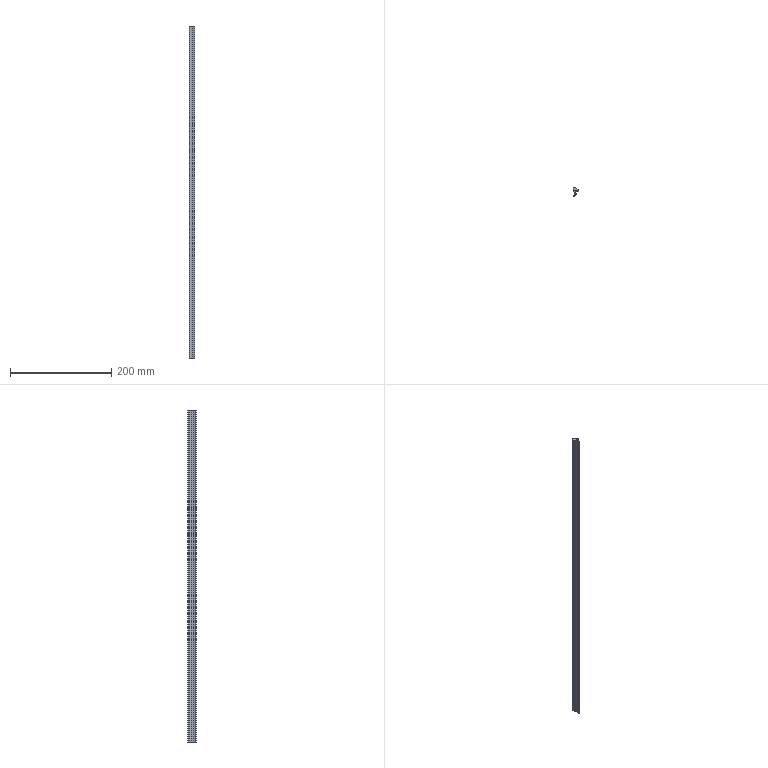Part | SolidWorks | features BaseBody 1, MoveFace 1 | 1 solid | 20 faces | box 10.8 x 17.5 x 657 mm | volume 51772 mm3 | cylinder 11 | plane 9 | commonest cylinder face diameters 1.6 x2 14 x2 0.4 x1 0.6 x1 0.8 x1 2.6 x1
STEP:
#1=CARTESIAN_POINT('',(-3.236,-11.055,557.));
#2=VERTEX_POINT('',#1);
#3=CARTESIAN_POINT('',(-4.3,-10.3,557.));
#4=VERTEX_POINT('',#3);
#5=CARTESIAN_POINT('',(-3.5,-10.3,557.));
#6=DIRECTION('',(0.,0.,-1.));
#7=DIRECTION('',(1.,0.,0.));
#8=AXIS2_PLACEMENT_3D('',#5,#6,#7);
#9=CIRCLE('',#8,0.8);
#10=EDGE_CURVE('',#2,#4,#9,.T.);
#11=ORIENTED_EDGE('',*,*,#10,.T.);
#12=CARTESIAN_POINT('',(-4.3,-10.3,-100.));
#13=VERTEX_POINT('',#12);
#14=CARTESIAN_POINT('',(-4.3,-10.3,-100.));
#15=DIRECTION('',(0.,0.,-1.));
#16=VECTOR('',#15,1000.);
#17=LINE('',#14,#16);
#18=EDGE_CURVE('',#4,#13,#17,.T.);
#19=ORIENTED_EDGE('',*,*,#18,.T.);
#20=CARTESIAN_POINT('',(-3.236,-11.055,-100.));
#21=VERTEX_POINT('',#20);
#22=CARTESIAN_POINT('',(-3.5,-10.3,-100.));
#23=DIRECTION('',(0.,0.,1.));
#24=DIRECTION('',(-1.,0.,0.));
#25=AXIS2_PLACEMENT_3D('',#22,#23,#24);
#26=CIRCLE('',#25,0.8);
#27=EDGE_CURVE('',#13,#21,#26,.T.);
#28=ORIENTED_EDGE('',*,*,#27,.T.);
#29=CARTESIAN_POINT('',(-3.236,-11.055,-100.));
#30=DIRECTION('',(0.,0.,-1.));
#31=VECTOR('',#30,1000.);
#32=LINE('',#29,#31);
#33=EDGE_CURVE('',#2,#21,#32,.T.);
#34=ORIENTED_EDGE('',*,*,#33,.F.);
#35=EDGE_LOOP('',(#11,#19,#28,#34));
#36=FACE_OUTER_BOUND('',#35,.T.);
#37=CARTESIAN_POINT('',(-3.5,-10.3,-100.));
#38=DIRECTION('',(0.,0.,-1.));
#39=DIRECTION('',(-1.,0.,0.));
#40=AXIS2_PLACEMENT_3D('',#37,#38,#39);
#41=CYLINDRICAL_SURFACE('',#40,0.8);
#42=ADVANCED_FACE('',(#36),#41,.T.);
#43=CARTESIAN_POINT('',(1.184,-6.397,-100.));
#44=VERTEX_POINT('',#43);
#45=CARTESIAN_POINT('',(-5.702,-4.29,-100.));
#46=DIRECTION('',(0.,0.,1.));
#47=DIRECTION('',(-1.,0.,0.));
#48=AXIS2_PLACEMENT_3D('',#45,#46,#47);
#49=CIRCLE('',#48,7.201);
#50=EDGE_CURVE('',#21,#44,#49,.T.);
#51=ORIENTED_EDGE('',*,*,#50,.T.);
#52=CARTESIAN_POINT('',(1.184,-6.397,557.));
#53=VERTEX_POINT('',#52);
#54=CARTESIAN_POINT('',(1.184,-6.397,-100.));
#55=DIRECTION('',(0.,0.,1.));
#56=VECTOR('',#55,1000.);
#57=LINE('',#54,#56);
#58=EDGE_CURVE('',#44,#53,#57,.T.);
#59=ORIENTED_EDGE('',*,*,#58,.T.);
#60=CARTESIAN_POINT('',(-5.702,-4.29,557.));
#61=DIRECTION('',(0.,0.,-1.));
#62=DIRECTION('',(1.,0.,0.));
#63=AXIS2_PLACEMENT_3D('',#60,#61,#62);
#64=CIRCLE('',#63,7.201);
#65=EDGE_CURVE('',#53,#2,#64,.T.);
#66=ORIENTED_EDGE('',*,*,#65,.T.);
#67=ORIENTED_EDGE('',*,*,#33,.T.);
#68=EDGE_LOOP('',(#51,#59,#66,#67));
#69=FACE_OUTER_BOUND('',#68,.T.);
#70=CARTESIAN_POINT('',(-5.702,-4.29,-100.));
#71=DIRECTION('',(0.,0.,-1.));
#72=DIRECTION('',(-1.,0.,0.));
#73=AXIS2_PLACEMENT_3D('',#70,#71,#72);
#74=CYLINDRICAL_SURFACE('',#73,7.201);
#75=ADVANCED_FACE('',(#69),#74,.T.);
#76=CARTESIAN_POINT('',(0.9,-6.,-100.));
#77=VERTEX_POINT('',#76);
#78=CARTESIAN_POINT('',(0.9,-6.3,-100.));
#79=DIRECTION('',(0.,0.,1.));
#80=DIRECTION('',(-1.,0.,0.));
#81=AXIS2_PLACEMENT_3D('',#78,#79,#80);
#82=CIRCLE('',#81,0.3);
#83=EDGE_CURVE('',#44,#77,#82,.T.);
#84=ORIENTED_EDGE('',*,*,#83,.T.);
#85=CARTESIAN_POINT('',(0.9,-6.,557.));
#86=VERTEX_POINT('',#85);
#87=CARTESIAN_POINT('',(0.9,-6.,-100.));
#88=DIRECTION('',(0.,0.,1.));
#89=VECTOR('',#88,1000.);
#90=LINE('',#87,#89);
#91=EDGE_CURVE('',#77,#86,#90,.T.);
#92=ORIENTED_EDGE('',*,*,#91,.T.);
#93=CARTESIAN_POINT('',(0.9,-6.3,557.));
#94=DIRECTION('',(0.,0.,-1.));
#95=DIRECTION('',(1.,0.,0.));
#96=AXIS2_PLACEMENT_3D('',#93,#94,#95);
#97=CIRCLE('',#96,0.3);
#98=EDGE_CURVE('',#86,#53,#97,.T.);
#99=ORIENTED_EDGE('',*,*,#98,.T.);
#100=ORIENTED_EDGE('',*,*,#58,.F.);
#101=EDGE_LOOP('',(#84,#92,#99,#100));
#102=FACE_OUTER_BOUND('',#101,.T.);
#103=CARTESIAN_POINT('',(0.9,-6.3,-100.));
#104=DIRECTION('',(0.,0.,-1.));
#105=DIRECTION('',(-1.,0.,0.));
#106=AXIS2_PLACEMENT_3D('',#103,#104,#105);
#107=CYLINDRICAL_SURFACE('',#106,0.3);
#108=ADVANCED_FACE('',(#102),#107,.T.);
#109=CARTESIAN_POINT('',(-2.5,-0.5,-100.));
#110=VERTEX_POINT('',#109);
#111=CARTESIAN_POINT('',(-2.5,-6.153,-100.));
#112=VERTEX_POINT('',#111);
#113=CARTESIAN_POINT('',(-2.5,-6.397,-100.));
#114=DIRECTION('',(0.,-1.,0.));
#115=VECTOR('',#114,1000.);
#116=LINE('',#113,#115);
#117=EDGE_CURVE('',#110,#112,#116,.T.);
#118=ORIENTED_EDGE('',*,*,#117,.F.);
#119=CARTESIAN_POINT('',(-4.2,1.695,-100.));
#120=VERTEX_POINT('',#119);
#121=CARTESIAN_POINT('',(-1.701,1.875,-100.));
#122=DIRECTION('',(0.,0.,1.));
#123=DIRECTION('',(-1.,0.,0.));
#124=AXIS2_PLACEMENT_3D('',#121,#122,#123);
#125=CIRCLE('',#124,2.506);
#126=EDGE_CURVE('',#120,#110,#125,.T.);
#127=ORIENTED_EDGE('',*,*,#126,.F.);
#128=CARTESIAN_POINT('',(-4.2,5.1,-100.));
#129=VERTEX_POINT('',#128);
#130=CARTESIAN_POINT('',(-4.2,-6.397,-100.));
#131=DIRECTION('',(0.,-1.,0.));
#132=VECTOR('',#131,1000.);
#133=LINE('',#130,#132);
#134=EDGE_CURVE('',#129,#120,#133,.T.);
#135=ORIENTED_EDGE('',*,*,#134,.F.);
#136=CARTESIAN_POINT('',(-2.892,6.4,-100.));
#137=VERTEX_POINT('',#136);
#138=CARTESIAN_POINT('',(-2.9,5.1,-100.));
#139=DIRECTION('',(0.,0.,1.));
#140=DIRECTION('',(-1.,0.,0.));
#141=AXIS2_PLACEMENT_3D('',#138,#139,#140);
#142=CIRCLE('',#141,1.3);
#143=EDGE_CURVE('',#137,#129,#142,.T.);
#144=ORIENTED_EDGE('',*,*,#143,.F.);
#145=CARTESIAN_POINT('',(0.5,5.5,-100.));
#146=VERTEX_POINT('',#145);
#147=CARTESIAN_POINT('',(-2.934,-0.5999,-100.));
#148=DIRECTION('',(0.,0.,1.));
#149=DIRECTION('',(-1.,0.,0.));
#150=AXIS2_PLACEMENT_3D('',#147,#148,#149);
#151=CIRCLE('',#150,7.);
#152=EDGE_CURVE('',#146,#137,#151,.T.);
#153=ORIENTED_EDGE('',*,*,#152,.F.);
#154=CARTESIAN_POINT('',(5.5,1.7,-100.));
#155=VERTEX_POINT('',#154);
#156=CARTESIAN_POINT('',(5.5,1.7,-100.));
#157=DIRECTION('',(-0.7962,0.6051,0.));
#158=VECTOR('',#157,1000.);
#159=LINE('',#156,#158);
#160=EDGE_CURVE('',#155,#146,#159,.T.);
#161=ORIENTED_EDGE('',*,*,#160,.F.);
#162=CARTESIAN_POINT('',(6.458,-0.2215,-100.));
#163=VERTEX_POINT('',#162);
#164=CARTESIAN_POINT('',(6.458,-0.2215,-100.));
#165=DIRECTION('',(-0.4462,0.8949,0.));
#166=VECTOR('',#165,1000.);
#167=LINE('',#164,#166);
#168=EDGE_CURVE('',#163,#155,#167,.T.);
#169=ORIENTED_EDGE('',*,*,#168,.F.);
#170=CARTESIAN_POINT('',(5.895,-0.7433,-100.));
#171=VERTEX_POINT('',#170);
#172=CARTESIAN_POINT('',(6.1,-0.4,-100.));
#173=DIRECTION('',(0.,0.,1.));
#174=DIRECTION('',(-1.,0.,0.));
#175=AXIS2_PLACEMENT_3D('',#172,#173,#174);
#176=CIRCLE('',#175,0.4);
#177=EDGE_CURVE('',#171,#163,#176,.T.);
#178=ORIENTED_EDGE('',*,*,#177,.F.);
#179=CARTESIAN_POINT('',(3.,0.,-100.));
#180=VERTEX_POINT('',#179);
#181=CARTESIAN_POINT('',(2.746,-6.995,-100.));
#182=DIRECTION('',(0.,0.,-1.));
#183=DIRECTION('',(-1.,0.,0.));
#184=AXIS2_PLACEMENT_3D('',#181,#182,#183);
#185=CIRCLE('',#184,7.);
#186=EDGE_CURVE('',#180,#171,#185,.T.);
#187=ORIENTED_EDGE('',*,*,#186,.F.);
#188=CARTESIAN_POINT('',(0.,0.,-100.));
#189=VERTEX_POINT('',#188);
#190=CARTESIAN_POINT('',(-6.814,0.,-100.));
#191=DIRECTION('',(1.,0.,0.));
#192=VECTOR('',#191,1000.);
#193=LINE('',#190,#192);
#194=EDGE_CURVE('',#189,#180,#193,.T.);
#195=ORIENTED_EDGE('',*,*,#194,.F.);
#196=CARTESIAN_POINT('',(0.,-5.8,-100.));
#197=VERTEX_POINT('',#196);
#198=CARTESIAN_POINT('',(0.,-6.397,-100.));
#199=DIRECTION('',(0.,1.,0.));
#200=VECTOR('',#199,1000.);
#201=LINE('',#198,#200);
#202=EDGE_CURVE('',#197,#189,#201,.T.);
#203=ORIENTED_EDGE('',*,*,#202,.F.);
#204=CARTESIAN_POINT('',(0.2,-6.,-100.));
#205=VERTEX_POINT('',#204);
#206=CARTESIAN_POINT('',(0.2,-5.8,-100.));
#207=DIRECTION('',(0.,0.,1.));
#208=DIRECTION('',(-1.,0.,0.));
#209=AXIS2_PLACEMENT_3D('',#206,#207,#208);
#210=CIRCLE('',#209,0.2);
#211=EDGE_CURVE('',#197,#205,#210,.T.);
#212=ORIENTED_EDGE('',*,*,#211,.T.);
#213=CARTESIAN_POINT('',(-6.814,-6.,-100.));
#214=DIRECTION('',(-1.,0.,0.));
#215=VECTOR('',#214,1000.);
#216=LINE('',#213,#215);
#217=EDGE_CURVE('',#77,#205,#216,.T.);
#218=ORIENTED_EDGE('',*,*,#217,.F.);
#219=ORIENTED_EDGE('',*,*,#83,.F.);
#220=ORIENTED_EDGE('',*,*,#50,.F.);
#221=ORIENTED_EDGE('',*,*,#27,.F.);
#222=CARTESIAN_POINT('',(-3.998,-9.674,-100.));
#223=VERTEX_POINT('',#222);
#224=CARTESIAN_POINT('',(-3.5,-10.3,-100.));
#225=DIRECTION('',(0.,0.,1.));
#226=DIRECTION('',(-1.,0.,0.));
#227=AXIS2_PLACEMENT_3D('',#224,#225,#226);
#228=CIRCLE('',#227,0.8);
#229=EDGE_CURVE('',#223,#13,#228,.T.);
#230=ORIENTED_EDGE('',*,*,#229,.F.);
#231=CARTESIAN_POINT('',(-6.814,-6.397,-100.));
#232=DIRECTION('',(0.,0.,-1.));
#233=DIRECTION('',(-1.,0.,0.));
#234=AXIS2_PLACEMENT_3D('',#231,#232,#233);
#235=CIRCLE('',#234,4.321);
#236=EDGE_CURVE('',#112,#223,#235,.T.);
#237=ORIENTED_EDGE('',*,*,#236,.F.);
#238=EDGE_LOOP('',(#118,#127,#135,#144,#153,#161,#169,#178,#187,#195,#203,#212,#218,#219,#220,#221,#230,#237));
#239=FACE_OUTER_BOUND('',#238,.T.);
#240=CARTESIAN_POINT('',(-6.814,-6.397,-100.));
#241=DIRECTION('',(0.,0.,1.));
#242=DIRECTION('',(1.,0.,0.));
#243=AXIS2_PLACEMENT_3D('',#240,#241,#242);
#244=PLANE('',#243);
#245=ADVANCED_FACE('',(#239),#244,.F.);
#246=ORIENTED_EDGE('',*,*,#18,.F.);
#247=CARTESIAN_POINT('',(-3.998,-9.674,557.));
#248=VERTEX_POINT('',#247);
#249=CARTESIAN_POINT('',(-3.5,-10.3,557.));
#250=DIRECTION('',(0.,0.,-1.));
#251=DIRECTION('',(1.,0.,0.));
#252=AXIS2_PLACEMENT_3D('',#249,#250,#251);
#253=CIRCLE('',#252,0.8);
#254=EDGE_CURVE('',#4,#248,#253,.T.);
#255=ORIENTED_EDGE('',*,*,#254,.T.);
#256=CARTESIAN_POINT('',(-3.998,-9.674,-100.));
#257=DIRECTION('',(0.,0.,-1.));
#258=VECTOR('',#257,1000.);
#259=LINE('',#256,#258);
#260=EDGE_CURVE('',#248,#223,#259,.T.);
#261=ORIENTED_EDGE('',*,*,#260,.T.);
#262=ORIENTED_EDGE('',*,*,#229,.T.);
#263=EDGE_LOOP('',(#246,#255,#261,#262));
#264=FACE_OUTER_BOUND('',#263,.T.);
#265=CARTESIAN_POINT('',(-3.5,-10.3,-100.));
#266=DIRECTION('',(0.,0.,-1.));
#267=DIRECTION('',(-1.,0.,0.));
#268=AXIS2_PLACEMENT_3D('',#265,#266,#267);
#269=CYLINDRICAL_SURFACE('',#268,0.8);
#270=ADVANCED_FACE('',(#264),#269,.T.);
#271=CARTESIAN_POINT('',(-4.2,1.695,557.));
#272=VERTEX_POINT('',#271);
#273=CARTESIAN_POINT('',(-2.5,-0.5,557.));
#274=VERTEX_POINT('',#273);
#275=CARTESIAN_POINT('',(-1.701,1.875,557.));
#276=DIRECTION('',(0.,0.,1.));
#277=DIRECTION('',(1.,0.,0.));
#278=AXIS2_PLACEMENT_3D('',#275,#276,#277);
#279=CIRCLE('',#278,2.506);
#280=EDGE_CURVE('',#272,#274,#279,.T.);
#281=ORIENTED_EDGE('',*,*,#280,.T.);
#282=CARTESIAN_POINT('',(-2.5,-6.153,557.));
#283=VERTEX_POINT('',#282);
#284=CARTESIAN_POINT('',(-2.5,-6.397,557.));
#285=DIRECTION('',(0.,-1.,0.));
#286=VECTOR('',#285,1000.);
#287=LINE('',#284,#286);
#288=EDGE_CURVE('',#274,#283,#287,.T.);
#289=ORIENTED_EDGE('',*,*,#288,.T.);
#290=CARTESIAN_POINT('',(-6.814,-6.397,557.));
#291=DIRECTION('',(0.,0.,-1.));
#292=DIRECTION('',(1.,0.,0.));
#293=AXIS2_PLACEMENT_3D('',#290,#291,#292);
#294=CIRCLE('',#293,4.321);
#295=EDGE_CURVE('',#283,#248,#294,.T.);
#296=ORIENTED_EDGE('',*,*,#295,.T.);
#297=ORIENTED_EDGE('',*,*,#254,.F.);
#298=ORIENTED_EDGE('',*,*,#10,.F.);
#299=ORIENTED_EDGE('',*,*,#65,.F.);
#300=ORIENTED_EDGE('',*,*,#98,.F.);
#301=CARTESIAN_POINT('',(0.2,-6.,557.));
#302=VERTEX_POINT('',#301);
#303=CARTESIAN_POINT('',(-6.814,-6.,557.));
#304=DIRECTION('',(-1.,0.,0.));
#305=VECTOR('',#304,1000.);
#306=LINE('',#303,#305);
#307=EDGE_CURVE('',#86,#302,#306,.T.);
#308=ORIENTED_EDGE('',*,*,#307,.T.);
#309=CARTESIAN_POINT('',(0.,-5.8,557.));
#310=VERTEX_POINT('',#309);
#311=CARTESIAN_POINT('',(0.2,-5.8,557.));
#312=DIRECTION('',(0.,0.,-1.));
#313=DIRECTION('',(1.,0.,0.));
#314=AXIS2_PLACEMENT_3D('',#311,#312,#313);
#315=CIRCLE('',#314,0.2);
#316=EDGE_CURVE('',#302,#310,#315,.T.);
#317=ORIENTED_EDGE('',*,*,#316,.T.);
#318=CARTESIAN_POINT('',(0.,0.,557.));
#319=VERTEX_POINT('',#318);
#320=CARTESIAN_POINT('',(0.,-6.397,557.));
#321=DIRECTION('',(0.,1.,0.));
#322=VECTOR('',#321,1000.);
#323=LINE('',#320,#322);
#324=EDGE_CURVE('',#310,#319,#323,.T.);
#325=ORIENTED_EDGE('',*,*,#324,.T.);
#326=CARTESIAN_POINT('',(3.,0.,557.));
#327=VERTEX_POINT('',#326);
#328=CARTESIAN_POINT('',(-6.814,0.,557.));
#329=DIRECTION('',(1.,0.,0.));
#330=VECTOR('',#329,1000.);
#331=LINE('',#328,#330);
#332=EDGE_CURVE('',#319,#327,#331,.T.);
#333=ORIENTED_EDGE('',*,*,#332,.T.);
#334=CARTESIAN_POINT('',(5.895,-0.7433,557.));
#335=VERTEX_POINT('',#334);
#336=CARTESIAN_POINT('',(2.746,-6.995,557.));
#337=DIRECTION('',(0.,0.,-1.));
#338=DIRECTION('',(1.,0.,0.));
#339=AXIS2_PLACEMENT_3D('',#336,#337,#338);
#340=CIRCLE('',#339,7.);
#341=EDGE_CURVE('',#327,#335,#340,.T.);
#342=ORIENTED_EDGE('',*,*,#341,.T.);
#343=CARTESIAN_POINT('',(6.458,-0.2215,557.));
#344=VERTEX_POINT('',#343);
#345=CARTESIAN_POINT('',(6.1,-0.4,557.));
#346=DIRECTION('',(0.,0.,-1.));
#347=DIRECTION('',(1.,0.,0.));
#348=AXIS2_PLACEMENT_3D('',#345,#346,#347);
#349=CIRCLE('',#348,0.4);
#350=EDGE_CURVE('',#344,#335,#349,.T.);
#351=ORIENTED_EDGE('',*,*,#350,.F.);
#352=CARTESIAN_POINT('',(5.5,1.7,557.));
#353=VERTEX_POINT('',#352);
#354=CARTESIAN_POINT('',(6.282,0.1323,557.));
#355=DIRECTION('',(-0.4462,0.8949,0.));
#356=VECTOR('',#355,1000.);
#357=LINE('',#354,#356);
#358=EDGE_CURVE('',#344,#353,#357,.T.);
#359=ORIENTED_EDGE('',*,*,#358,.T.);
#360=CARTESIAN_POINT('',(0.5,5.5,557.));
#361=VERTEX_POINT('',#360);
#362=CARTESIAN_POINT('',(1.595,4.668,557.));
#363=DIRECTION('',(-0.7962,0.6051,0.));
#364=VECTOR('',#363,1000.);
#365=LINE('',#362,#364);
#366=EDGE_CURVE('',#353,#361,#365,.T.);
#367=ORIENTED_EDGE('',*,*,#366,.T.);
#368=CARTESIAN_POINT('',(-2.892,6.4,557.));
#369=VERTEX_POINT('',#368);
#370=CARTESIAN_POINT('',(-2.934,-0.5999,557.));
#371=DIRECTION('',(0.,0.,1.));
#372=DIRECTION('',(1.,0.,0.));
#373=AXIS2_PLACEMENT_3D('',#370,#371,#372);
#374=CIRCLE('',#373,7.);
#375=EDGE_CURVE('',#361,#369,#374,.T.);
#376=ORIENTED_EDGE('',*,*,#375,.T.);
#377=CARTESIAN_POINT('',(-4.2,5.1,557.));
#378=VERTEX_POINT('',#377);
#379=CARTESIAN_POINT('',(-2.9,5.1,557.));
#380=DIRECTION('',(0.,0.,1.));
#381=DIRECTION('',(1.,0.,0.));
#382=AXIS2_PLACEMENT_3D('',#379,#380,#381);
#383=CIRCLE('',#382,1.3);
#384=EDGE_CURVE('',#369,#378,#383,.T.);
#385=ORIENTED_EDGE('',*,*,#384,.T.);
#386=CARTESIAN_POINT('',(-4.2,-6.397,557.));
#387=DIRECTION('',(0.,-1.,0.));
#388=VECTOR('',#387,1000.);
#389=LINE('',#386,#388);
#390=EDGE_CURVE('',#378,#272,#389,.T.);
#391=ORIENTED_EDGE('',*,*,#390,.T.);
#392=EDGE_LOOP('',(#281,#289,#296,#297,#298,#299,#300,#308,#317,#325,#333,#342,#351,#359,#367,#376,#385,#391));
#393=FACE_OUTER_BOUND('',#392,.T.);
#394=CARTESIAN_POINT('',(-6.814,-6.397,557.));
#395=DIRECTION('',(0.,0.,1.));
#396=DIRECTION('',(1.,0.,0.));
#397=AXIS2_PLACEMENT_3D('',#394,#395,#396);
#398=PLANE('',#397);
#399=ADVANCED_FACE('',(#393),#398,.T.);
#400=ORIENTED_EDGE('',*,*,#217,.T.);
#401=CARTESIAN_POINT('',(0.2,-6.,-100.));
#402=DIRECTION('',(0.,0.,1.));
#403=VECTOR('',#402,1000.);
#404=LINE('',#401,#403);
#405=EDGE_CURVE('',#205,#302,#404,.T.);
#406=ORIENTED_EDGE('',*,*,#405,.T.);
#407=ORIENTED_EDGE('',*,*,#307,.F.);
#408=ORIENTED_EDGE('',*,*,#91,.F.);
#409=EDGE_LOOP('',(#400,#406,#407,#408));
#410=FACE_OUTER_BOUND('',#409,.T.);
#411=CARTESIAN_POINT('',(0.9,-6.,-100.));
#412=DIRECTION('',(0.,1.,0.));
#413=DIRECTION('',(0.,0.,1.));
#414=AXIS2_PLACEMENT_3D('',#411,#412,#413);
#415=PLANE('',#414);
#416=ADVANCED_FACE('',(#410),#415,.T.);
#417=CARTESIAN_POINT('',(-2.5,-6.153,-100.));
#418=DIRECTION('',(0.,0.,1.));
#419=VECTOR('',#418,1000.);
#420=LINE('',#417,#419);
#421=EDGE_CURVE('',#112,#283,#420,.T.);
#422=ORIENTED_EDGE('',*,*,#421,.F.);
#423=ORIENTED_EDGE('',*,*,#236,.T.);
#424=ORIENTED_EDGE('',*,*,#260,.F.);
#425=ORIENTED_EDGE('',*,*,#295,.F.);
#426=EDGE_LOOP('',(#422,#423,#424,#425));
#427=FACE_OUTER_BOUND('',#426,.T.);
#428=CARTESIAN_POINT('',(-6.814,-6.397,-100.));
#429=DIRECTION('',(0.,0.,-1.));
#430=DIRECTION('',(-1.,0.,0.));
#431=AXIS2_PLACEMENT_3D('',#428,#429,#430);
#432=CYLINDRICAL_SURFACE('',#431,4.321);
#433=ADVANCED_FACE('',(#427),#432,.F.);
#434=ORIENTED_EDGE('',*,*,#117,.T.);
#435=ORIENTED_EDGE('',*,*,#421,.T.);
#436=ORIENTED_EDGE('',*,*,#288,.F.);
#437=CARTESIAN_POINT('',(-2.5,-0.5,-100.));
#438=DIRECTION('',(0.,0.,-1.));
#439=VECTOR('',#438,1000.);
#440=LINE('',#437,#439);
#441=EDGE_CURVE('',#274,#110,#440,.T.);
#442=ORIENTED_EDGE('',*,*,#441,.T.);
#443=EDGE_LOOP('',(#434,#435,#436,#442));
#444=FACE_OUTER_BOUND('',#443,.T.);
#445=CARTESIAN_POINT('',(-2.5,-0.5,-100.));
#446=DIRECTION('',(-1.,0.,0.));
#447=DIRECTION('',(0.,0.,1.));
#448=AXIS2_PLACEMENT_3D('',#445,#446,#447);
#449=PLANE('',#448);
#450=ADVANCED_FACE('',(#444),#449,.T.);
#451=ORIENTED_EDGE('',*,*,#126,.T.);
#452=ORIENTED_EDGE('',*,*,#441,.F.);
#453=ORIENTED_EDGE('',*,*,#280,.F.);
#454=CARTESIAN_POINT('',(-4.2,1.695,-100.));
#455=DIRECTION('',(0.,0.,-1.));
#456=VECTOR('',#455,1000.);
#457=LINE('',#454,#456);
#458=EDGE_CURVE('',#272,#120,#457,.T.);
#459=ORIENTED_EDGE('',*,*,#458,.T.);
#460=EDGE_LOOP('',(#451,#452,#453,#459));
#461=FACE_OUTER_BOUND('',#460,.T.);
#462=CARTESIAN_POINT('',(-1.701,1.875,-100.));
#463=DIRECTION('',(0.,0.,-1.));
#464=DIRECTION('',(-1.,0.,0.));
#465=AXIS2_PLACEMENT_3D('',#462,#463,#464);
#466=CYLINDRICAL_SURFACE('',#465,2.506);
#467=ADVANCED_FACE('',(#461),#466,.T.);
#468=ORIENTED_EDGE('',*,*,#134,.T.);
#469=ORIENTED_EDGE('',*,*,#458,.F.);
#470=ORIENTED_EDGE('',*,*,#390,.F.);
#471=CARTESIAN_POINT('',(-4.2,5.1,-100.));
#472=DIRECTION('',(0.,0.,-1.));
#473=VECTOR('',#472,1000.);
#474=LINE('',#471,#473);
#475=EDGE_CURVE('',#378,#129,#474,.T.);
#476=ORIENTED_EDGE('',*,*,#475,.T.);
#477=EDGE_LOOP('',(#468,#469,#470,#476));
#478=FACE_OUTER_BOUND('',#477,.T.);
#479=CARTESIAN_POINT('',(-4.2,5.1,-100.));
#480=DIRECTION('',(-1.,0.,0.));
#481=DIRECTION('',(0.,0.,1.));
#482=AXIS2_PLACEMENT_3D('',#479,#480,#481);
#483=PLANE('',#482);
#484=ADVANCED_FACE('',(#478),#483,.T.);
#485=ORIENTED_EDGE('',*,*,#143,.T.);
#486=ORIENTED_EDGE('',*,*,#475,.F.);
#487=ORIENTED_EDGE('',*,*,#384,.F.);
#488=CARTESIAN_POINT('',(-2.892,6.4,-100.));
#489=DIRECTION('',(0.,0.,-1.));
#490=VECTOR('',#489,1000.);
#491=LINE('',#488,#490);
#492=EDGE_CURVE('',#369,#137,#491,.T.);
#493=ORIENTED_EDGE('',*,*,#492,.T.);
#494=EDGE_LOOP('',(#485,#486,#487,#493));
#495=FACE_OUTER_BOUND('',#494,.T.);
#496=CARTESIAN_POINT('',(-2.9,5.1,-100.));
#497=DIRECTION('',(0.,0.,-1.));
#498=DIRECTION('',(-1.,0.,0.));
#499=AXIS2_PLACEMENT_3D('',#496,#497,#498);
#500=CYLINDRICAL_SURFACE('',#499,1.3);
#501=ADVANCED_FACE('',(#495),#500,.T.);
#502=ORIENTED_EDGE('',*,*,#152,.T.);
#503=ORIENTED_EDGE('',*,*,#492,.F.);
#504=ORIENTED_EDGE('',*,*,#375,.F.);
#505=CARTESIAN_POINT('',(0.5,5.5,-100.));
#506=DIRECTION('',(0.,0.,-1.));
#507=VECTOR('',#506,1000.);
#508=LINE('',#505,#507);
#509=EDGE_CURVE('',#361,#146,#508,.T.);
#510=ORIENTED_EDGE('',*,*,#509,.T.);
#511=EDGE_LOOP('',(#502,#503,#504,#510));
#512=FACE_OUTER_BOUND('',#511,.T.);
#513=CARTESIAN_POINT('',(-2.934,-0.5999,-100.));
#514=DIRECTION('',(0.,0.,-1.));
#515=DIRECTION('',(-1.,0.,0.));
#516=AXIS2_PLACEMENT_3D('',#513,#514,#515);
#517=CYLINDRICAL_SURFACE('',#516,7.);
#518=ADVANCED_FACE('',(#512),#517,.T.);
#519=ORIENTED_EDGE('',*,*,#160,.T.);
#520=ORIENTED_EDGE('',*,*,#509,.F.);
#521=ORIENTED_EDGE('',*,*,#366,.F.);
#522=CARTESIAN_POINT('',(5.5,1.7,-100.));
#523=DIRECTION('',(0.,0.,-1.));
#524=VECTOR('',#523,1000.);
#525=LINE('',#522,#524);
#526=EDGE_CURVE('',#353,#155,#525,.T.);
#527=ORIENTED_EDGE('',*,*,#526,.T.);
#528=EDGE_LOOP('',(#519,#520,#521,#527));
#529=FACE_OUTER_BOUND('',#528,.T.);
#530=CARTESIAN_POINT('',(5.5,1.7,-100.));
#531=DIRECTION('',(0.6051,0.7962,0.));
#532=DIRECTION('',(-0.7962,0.6051,0.));
#533=AXIS2_PLACEMENT_3D('',#530,#531,#532);
#534=PLANE('',#533);
#535=ADVANCED_FACE('',(#529),#534,.T.);
#536=ORIENTED_EDGE('',*,*,#168,.T.);
#537=ORIENTED_EDGE('',*,*,#526,.F.);
#538=ORIENTED_EDGE('',*,*,#358,.F.);
#539=CARTESIAN_POINT('',(6.458,-0.2215,-100.));
#540=DIRECTION('',(0.,0.,-1.));
#541=VECTOR('',#540,1000.);
#542=LINE('',#539,#541);
#543=EDGE_CURVE('',#344,#163,#542,.T.);
#544=ORIENTED_EDGE('',*,*,#543,.T.);
#545=EDGE_LOOP('',(#536,#537,#538,#544));
#546=FACE_OUTER_BOUND('',#545,.T.);
#547=CARTESIAN_POINT('',(6.458,-0.2215,-100.));
#548=DIRECTION('',(0.8949,0.4462,0.));
#549=DIRECTION('',(-0.4462,0.8949,0.));
#550=AXIS2_PLACEMENT_3D('',#547,#548,#549);
#551=PLANE('',#550);
#552=ADVANCED_FACE('',(#546),#551,.T.);
#553=CARTESIAN_POINT('',(3.,0.,-100.));
#554=DIRECTION('',(0.,0.,1.));
#555=VECTOR('',#554,1000.);
#556=LINE('',#553,#555);
#557=EDGE_CURVE('',#180,#327,#556,.T.);
#558=ORIENTED_EDGE('',*,*,#557,.F.);
#559=ORIENTED_EDGE('',*,*,#186,.T.);
#560=CARTESIAN_POINT('',(5.895,-0.7433,-100.));
#561=DIRECTION('',(0.,0.,-1.));
#562=VECTOR('',#561,1000.);
#563=LINE('',#560,#562);
#564=EDGE_CURVE('',#335,#171,#563,.T.);
#565=ORIENTED_EDGE('',*,*,#564,.F.);
#566=ORIENTED_EDGE('',*,*,#341,.F.);
#567=EDGE_LOOP('',(#558,#559,#565,#566));
#568=FACE_OUTER_BOUND('',#567,.T.);
#569=CARTESIAN_POINT('',(2.746,-6.995,-100.));
#570=DIRECTION('',(0.,0.,-1.));
#571=DIRECTION('',(-1.,0.,0.));
#572=AXIS2_PLACEMENT_3D('',#569,#570,#571);
#573=CYLINDRICAL_SURFACE('',#572,7.);
#574=ADVANCED_FACE('',(#568),#573,.F.);
#575=ORIENTED_EDGE('',*,*,#194,.T.);
#576=ORIENTED_EDGE('',*,*,#557,.T.);
#577=ORIENTED_EDGE('',*,*,#332,.F.);
#578=CARTESIAN_POINT('',(0.,0.,-100.));
#579=DIRECTION('',(0.,0.,-1.));
#580=VECTOR('',#579,1000.);
#581=LINE('',#578,#580);
#582=EDGE_CURVE('',#319,#189,#581,.T.);
#583=ORIENTED_EDGE('',*,*,#582,.T.);
#584=EDGE_LOOP('',(#575,#576,#577,#583));
#585=FACE_OUTER_BOUND('',#584,.T.);
#586=CARTESIAN_POINT('',(0.,0.,-100.));
#587=DIRECTION('',(0.,-1.,0.));
#588=DIRECTION('',(0.,0.,-1.));
#589=AXIS2_PLACEMENT_3D('',#586,#587,#588);
#590=PLANE('',#589);
#591=ADVANCED_FACE('',(#585),#590,.T.);
#592=ORIENTED_EDGE('',*,*,#202,.T.);
#593=ORIENTED_EDGE('',*,*,#582,.F.);
#594=ORIENTED_EDGE('',*,*,#324,.F.);
#595=CARTESIAN_POINT('',(0.,-5.8,-100.));
#596=DIRECTION('',(0.,0.,-1.));
#597=VECTOR('',#596,1000.);
#598=LINE('',#595,#597);
#599=EDGE_CURVE('',#310,#197,#598,.T.);
#600=ORIENTED_EDGE('',*,*,#599,.T.);
#601=EDGE_LOOP('',(#592,#593,#594,#600));
#602=FACE_OUTER_BOUND('',#601,.T.);
#603=CARTESIAN_POINT('',(0.,-5.8,-100.));
#604=DIRECTION('',(1.,0.,0.));
#605=DIRECTION('',(0.,0.,-1.));
#606=AXIS2_PLACEMENT_3D('',#603,#604,#605);
#607=PLANE('',#606);
#608=ADVANCED_FACE('',(#602),#607,.T.);
#609=ORIENTED_EDGE('',*,*,#405,.F.);
#610=ORIENTED_EDGE('',*,*,#211,.F.);
#611=ORIENTED_EDGE('',*,*,#599,.F.);
#612=ORIENTED_EDGE('',*,*,#316,.F.);
#613=EDGE_LOOP('',(#609,#610,#611,#612));
#614=FACE_OUTER_BOUND('',#613,.T.);
#615=CARTESIAN_POINT('',(0.2,-5.8,-100.));
#616=DIRECTION('',(0.,0.,-1.));
#617=DIRECTION('',(-1.,0.,0.));
#618=AXIS2_PLACEMENT_3D('',#615,#616,#617);
#619=CYLINDRICAL_SURFACE('',#618,0.2);
#620=ADVANCED_FACE('',(#614),#619,.F.);
#621=ORIENTED_EDGE('',*,*,#177,.T.);
#622=ORIENTED_EDGE('',*,*,#543,.F.);
#623=ORIENTED_EDGE('',*,*,#350,.T.);
#624=ORIENTED_EDGE('',*,*,#564,.T.);
#625=EDGE_LOOP('',(#621,#622,#623,#624));
#626=FACE_OUTER_BOUND('',#625,.T.);
#627=CARTESIAN_POINT('',(6.1,-0.4,-100.));
#628=DIRECTION('',(0.,0.,-1.));
#629=DIRECTION('',(-1.,0.,0.));
#630=AXIS2_PLACEMENT_3D('',#627,#628,#629);
#631=CYLINDRICAL_SURFACE('',#630,0.4);
#632=ADVANCED_FACE('',(#626),#631,.T.);
#633=CLOSED_SHELL('',(#42,#75,#108,#245,#270,#399,#416,#433,#450,#467,#484,#501,#518,#535,#552,#574,#591,#608,#620,#632));
#634=MANIFOLD_SOLID_BREP('',#633);
#635=CARTESIAN_POINT('',(0.,0.,0.));
#636=DIRECTION('',(0.,0.,1.));
#637=DIRECTION('',(1.,0.,0.));
#638=AXIS2_PLACEMENT_3D('',#635,#636,#637);
#639=(LENGTH_UNIT()NAMED_UNIT(*)SI_UNIT(.MILLI.,.METRE.));
#640=UNCERTAINTY_MEASURE_WITH_UNIT(LENGTH_MEASURE(0.00001),#639,'','');
#641=(NAMED_UNIT(*)PLANE_ANGLE_UNIT()SI_UNIT($,.RADIAN.));
#642=(NAMED_UNIT(*)SI_UNIT($,.STERADIAN.)SOLID_ANGLE_UNIT());
#643=(GEOMETRIC_REPRESENTATION_CONTEXT(3)GLOBAL_UNCERTAINTY_ASSIGNED_CONTEXT((#640))GLOBAL_UNIT_ASSIGNED_CONTEXT((#639,#641,#642))REPRESENTATION_CONTEXT('',''));
#644=ADVANCED_BREP_SHAPE_REPRESENTATION('',(#634,#638),#643);